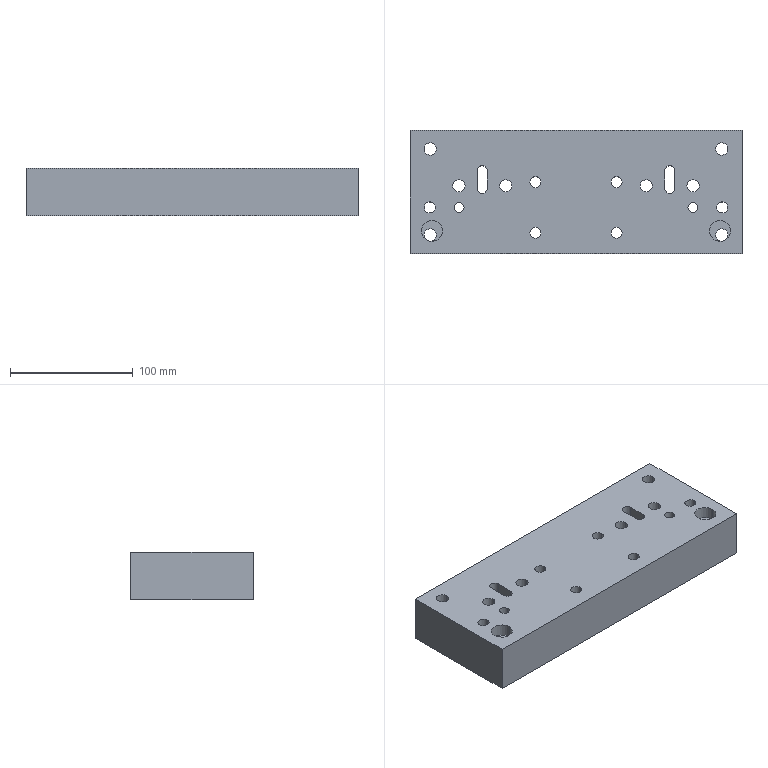Part | STEP file | TAM DE COI | 1 solid | 72 faces | box 270 x 100 x 39 mm | volume 987341 mm3 | cylinder 54 | plane 18 | commonest cylinder face diameters 9 x12 15 x12 8 x8 10 x8 10.106 x8 16.99 x6